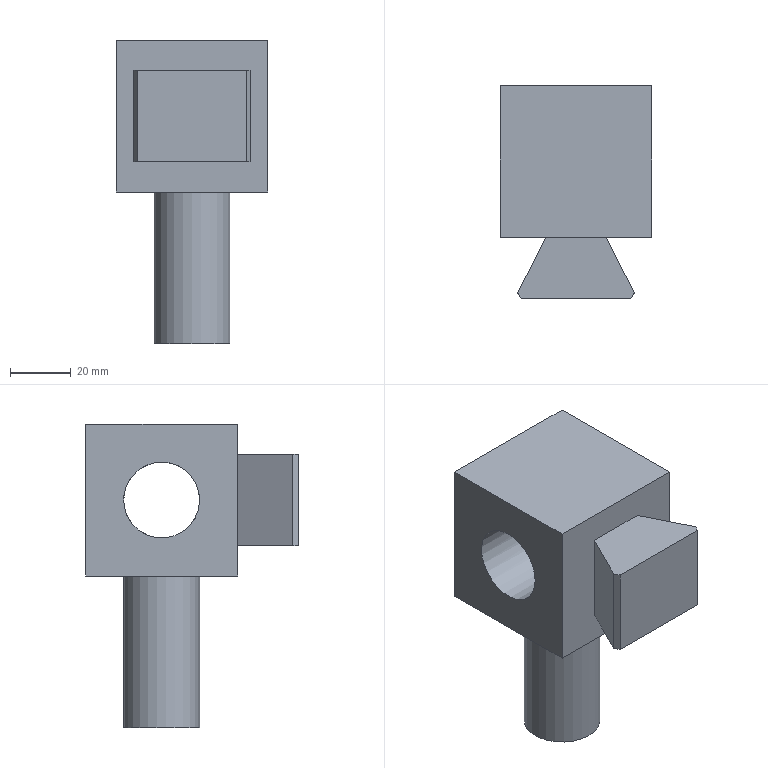Part | NX | features DATUM_CSYS 4, EXTRUDE 4, SKETCH 3, CHAMFER 1 | 1 solid | 16 faces | box 50 x 70 x 100 mm | volume 142893 mm3 | plane 14 | cylinder 2 | commonest cylinder face diameters 25 x2
STEP:
#1=CARTESIAN_POINT('',(-25.,0.,12.5));
#2=VERTEX_POINT('',#1);
#3=CARTESIAN_POINT('',(-25.,0.,0.));
#4=DIRECTION('',(-1.,0.,0.));
#5=DIRECTION('',(0.,0.,1.));
#6=AXIS2_PLACEMENT_3D('',#3,#4,#5);
#7=CIRCLE('',#6,12.5);
#8=EDGE_CURVE('',#2,#2,#7,.T.);
#9=ORIENTED_EDGE('',*,*,#8,.F.);
#10=EDGE_LOOP('',(#9));
#11=FACE_BOUND('',#10,.T.);
#12=CARTESIAN_POINT('',(-25.,25.,-25.));
#13=VERTEX_POINT('',#12);
#14=CARTESIAN_POINT('',(-25.,-25.,-25.));
#15=VERTEX_POINT('',#14);
#16=CARTESIAN_POINT('',(-25.,25.,-25.));
#17=DIRECTION('',(0.,-1.,0.));
#18=VECTOR('',#17,1000.);
#19=LINE('',#16,#18);
#20=EDGE_CURVE('',#13,#15,#19,.T.);
#21=ORIENTED_EDGE('',*,*,#20,.T.);
#22=CARTESIAN_POINT('',(-25.,-25.,25.));
#23=VERTEX_POINT('',#22);
#24=CARTESIAN_POINT('',(-25.,-25.,25.));
#25=DIRECTION('',(0.,0.,-1.));
#26=VECTOR('',#25,1000.);
#27=LINE('',#24,#26);
#28=EDGE_CURVE('',#23,#15,#27,.T.);
#29=ORIENTED_EDGE('',*,*,#28,.F.);
#30=CARTESIAN_POINT('',(-25.,25.,25.));
#31=VERTEX_POINT('',#30);
#32=CARTESIAN_POINT('',(-25.,25.,25.));
#33=DIRECTION('',(0.,-1.,0.));
#34=VECTOR('',#33,1000.);
#35=LINE('',#32,#34);
#36=EDGE_CURVE('',#31,#23,#35,.T.);
#37=ORIENTED_EDGE('',*,*,#36,.F.);
#38=CARTESIAN_POINT('',(-25.,25.,25.));
#39=DIRECTION('',(0.,0.,-1.));
#40=VECTOR('',#39,1000.);
#41=LINE('',#38,#40);
#42=EDGE_CURVE('',#31,#13,#41,.T.);
#43=ORIENTED_EDGE('',*,*,#42,.T.);
#44=EDGE_LOOP('',(#21,#29,#37,#43));
#45=FACE_BOUND('',#44,.T.);
#46=CARTESIAN_POINT('',(-25.,25.,25.));
#47=DIRECTION('',(1.,0.,0.));
#48=DIRECTION('',(0.,1.,0.));
#49=AXIS2_PLACEMENT_3D('',#46,#47,#48);
#50=PLANE('',#49);
#51=ADVANCED_FACE('',(#11,#45),#50,.F.);
#52=CARTESIAN_POINT('',(10.,-25.,15.));
#53=VERTEX_POINT('',#52);
#54=CARTESIAN_POINT('',(10.,-25.,-15.));
#55=VERTEX_POINT('',#54);
#56=CARTESIAN_POINT('',(10.,-25.,15.));
#57=DIRECTION('',(0.,0.,-1.));
#58=VECTOR('',#57,1000.);
#59=LINE('',#56,#58);
#60=EDGE_CURVE('',#53,#55,#59,.T.);
#61=ORIENTED_EDGE('',*,*,#60,.T.);
#62=CARTESIAN_POINT('',(-10.,-25.,-15.));
#63=VERTEX_POINT('',#62);
#64=CARTESIAN_POINT('',(10.,-25.,-15.));
#65=DIRECTION('',(-1.,0.,0.));
#66=VECTOR('',#65,1000.);
#67=LINE('',#64,#66);
#68=EDGE_CURVE('',#55,#63,#67,.T.);
#69=ORIENTED_EDGE('',*,*,#68,.T.);
#70=CARTESIAN_POINT('',(-10.,-25.,15.));
#71=VERTEX_POINT('',#70);
#72=CARTESIAN_POINT('',(-10.,-25.,15.));
#73=DIRECTION('',(0.,0.,-1.));
#74=VECTOR('',#73,1000.);
#75=LINE('',#72,#74);
#76=EDGE_CURVE('',#71,#63,#75,.T.);
#77=ORIENTED_EDGE('',*,*,#76,.F.);
#78=CARTESIAN_POINT('',(10.,-25.,15.));
#79=DIRECTION('',(-1.,0.,0.));
#80=VECTOR('',#79,1000.);
#81=LINE('',#78,#80);
#82=EDGE_CURVE('',#53,#71,#81,.T.);
#83=ORIENTED_EDGE('',*,*,#82,.F.);
#84=EDGE_LOOP('',(#61,#69,#77,#83));
#85=FACE_BOUND('',#84,.T.);
#86=CARTESIAN_POINT('',(25.,-25.,-25.));
#87=VERTEX_POINT('',#86);
#88=CARTESIAN_POINT('',(-25.,-25.,-25.));
#89=DIRECTION('',(1.,0.,0.));
#90=VECTOR('',#89,1000.);
#91=LINE('',#88,#90);
#92=EDGE_CURVE('',#15,#87,#91,.T.);
#93=ORIENTED_EDGE('',*,*,#92,.T.);
#94=CARTESIAN_POINT('',(25.,-25.,25.));
#95=VERTEX_POINT('',#94);
#96=CARTESIAN_POINT('',(25.,-25.,25.));
#97=DIRECTION('',(0.,0.,-1.));
#98=VECTOR('',#97,1000.);
#99=LINE('',#96,#98);
#100=EDGE_CURVE('',#95,#87,#99,.T.);
#101=ORIENTED_EDGE('',*,*,#100,.F.);
#102=CARTESIAN_POINT('',(-25.,-25.,25.));
#103=DIRECTION('',(1.,0.,0.));
#104=VECTOR('',#103,1000.);
#105=LINE('',#102,#104);
#106=EDGE_CURVE('',#23,#95,#105,.T.);
#107=ORIENTED_EDGE('',*,*,#106,.F.);
#108=ORIENTED_EDGE('',*,*,#28,.T.);
#109=EDGE_LOOP('',(#93,#101,#107,#108));
#110=FACE_BOUND('',#109,.T.);
#111=CARTESIAN_POINT('',(-25.,-25.,25.));
#112=DIRECTION('',(0.,1.,0.));
#113=DIRECTION('',(-1.,0.,0.));
#114=AXIS2_PLACEMENT_3D('',#111,#112,#113);
#115=PLANE('',#114);
#116=ADVANCED_FACE('',(#85,#110),#115,.F.);
#117=CARTESIAN_POINT('',(25.,-12.5,0.));
#118=VERTEX_POINT('',#117);
#119=CARTESIAN_POINT('',(25.,0.,0.));
#120=DIRECTION('',(-1.,0.,0.));
#121=DIRECTION('',(0.,-1.,0.));
#122=AXIS2_PLACEMENT_3D('',#119,#120,#121);
#123=CIRCLE('',#122,12.5);
#124=EDGE_CURVE('',#118,#118,#123,.T.);
#125=ORIENTED_EDGE('',*,*,#124,.T.);
#126=EDGE_LOOP('',(#125));
#127=FACE_BOUND('',#126,.T.);
#128=CARTESIAN_POINT('',(25.,25.,-25.));
#129=VERTEX_POINT('',#128);
#130=CARTESIAN_POINT('',(25.,-25.,-25.));
#131=DIRECTION('',(0.,1.,0.));
#132=VECTOR('',#131,1000.);
#133=LINE('',#130,#132);
#134=EDGE_CURVE('',#87,#129,#133,.T.);
#135=ORIENTED_EDGE('',*,*,#134,.T.);
#136=CARTESIAN_POINT('',(25.,25.,25.));
#137=VERTEX_POINT('',#136);
#138=CARTESIAN_POINT('',(25.,25.,25.));
#139=DIRECTION('',(0.,0.,-1.));
#140=VECTOR('',#139,1000.);
#141=LINE('',#138,#140);
#142=EDGE_CURVE('',#137,#129,#141,.T.);
#143=ORIENTED_EDGE('',*,*,#142,.F.);
#144=CARTESIAN_POINT('',(25.,-25.,25.));
#145=DIRECTION('',(0.,1.,0.));
#146=VECTOR('',#145,1000.);
#147=LINE('',#144,#146);
#148=EDGE_CURVE('',#95,#137,#147,.T.);
#149=ORIENTED_EDGE('',*,*,#148,.F.);
#150=ORIENTED_EDGE('',*,*,#100,.T.);
#151=EDGE_LOOP('',(#135,#143,#149,#150));
#152=FACE_BOUND('',#151,.T.);
#153=CARTESIAN_POINT('',(25.,-25.,25.));
#154=DIRECTION('',(-1.,0.,0.));
#155=DIRECTION('',(0.,-1.,0.));
#156=AXIS2_PLACEMENT_3D('',#153,#154,#155);
#157=PLANE('',#156);
#158=ADVANCED_FACE('',(#127,#152),#157,.F.);
#159=CARTESIAN_POINT('',(25.,25.,-25.));
#160=DIRECTION('',(-1.,0.,0.));
#161=VECTOR('',#160,1000.);
#162=LINE('',#159,#161);
#163=EDGE_CURVE('',#129,#13,#162,.T.);
#164=ORIENTED_EDGE('',*,*,#163,.T.);
#165=ORIENTED_EDGE('',*,*,#42,.F.);
#166=CARTESIAN_POINT('',(25.,25.,25.));
#167=DIRECTION('',(-1.,0.,0.));
#168=VECTOR('',#167,1000.);
#169=LINE('',#166,#168);
#170=EDGE_CURVE('',#137,#31,#169,.T.);
#171=ORIENTED_EDGE('',*,*,#170,.F.);
#172=ORIENTED_EDGE('',*,*,#142,.T.);
#173=EDGE_LOOP('',(#164,#165,#171,#172));
#174=FACE_BOUND('',#173,.T.);
#175=CARTESIAN_POINT('',(25.,25.,25.));
#176=DIRECTION('',(0.,-1.,0.));
#177=DIRECTION('',(0.,0.,-1.));
#178=AXIS2_PLACEMENT_3D('',#175,#176,#177);
#179=PLANE('',#178);
#180=ADVANCED_FACE('',(#174),#179,.F.);
#181=ORIENTED_EDGE('',*,*,#36,.T.);
#182=ORIENTED_EDGE('',*,*,#106,.T.);
#183=ORIENTED_EDGE('',*,*,#148,.T.);
#184=ORIENTED_EDGE('',*,*,#170,.T.);
#185=EDGE_LOOP('',(#181,#182,#183,#184));
#186=FACE_BOUND('',#185,.T.);
#187=CARTESIAN_POINT('',(0.,0.,25.));
#188=DIRECTION('',(0.,0.,1.));
#189=DIRECTION('',(1.,0.,0.));
#190=AXIS2_PLACEMENT_3D('',#187,#188,#189);
#191=PLANE('',#190);
#192=ADVANCED_FACE('',(#186),#191,.T.);
#193=CARTESIAN_POINT('',(0.,12.5,-25.));
#194=VERTEX_POINT('',#193);
#195=CARTESIAN_POINT('',(0.,0.,-25.));
#196=DIRECTION('',(0.,0.,-1.));
#197=DIRECTION('',(0.,1.,0.));
#198=AXIS2_PLACEMENT_3D('',#195,#196,#197);
#199=CIRCLE('',#198,12.5);
#200=EDGE_CURVE('',#194,#194,#199,.T.);
#201=ORIENTED_EDGE('',*,*,#200,.F.);
#202=EDGE_LOOP('',(#201));
#203=FACE_BOUND('',#202,.T.);
#204=ORIENTED_EDGE('',*,*,#20,.F.);
#205=ORIENTED_EDGE('',*,*,#163,.F.);
#206=ORIENTED_EDGE('',*,*,#134,.F.);
#207=ORIENTED_EDGE('',*,*,#92,.F.);
#208=EDGE_LOOP('',(#204,#205,#206,#207));
#209=FACE_BOUND('',#208,.T.);
#210=CARTESIAN_POINT('',(0.,0.,-25.));
#211=DIRECTION('',(0.,0.,1.));
#212=DIRECTION('',(1.,0.,0.));
#213=AXIS2_PLACEMENT_3D('',#210,#211,#212);
#214=PLANE('',#213);
#215=ADVANCED_FACE('',(#203,#209),#214,.F.);
#216=CARTESIAN_POINT('',(-19.106,-43.211,-15.));
#217=VERTEX_POINT('',#216);
#218=CARTESIAN_POINT('',(-10.,-25.,-15.));
#219=DIRECTION('',(-0.4472,-0.8944,0.));
#220=VECTOR('',#219,1000.);
#221=LINE('',#218,#220);
#222=EDGE_CURVE('',#63,#217,#221,.T.);
#223=ORIENTED_EDGE('',*,*,#222,.T.);
#224=CARTESIAN_POINT('',(-19.106,-43.211,15.));
#225=VERTEX_POINT('',#224);
#226=CARTESIAN_POINT('',(-19.106,-43.211,15.));
#227=DIRECTION('',(0.,0.,1.));
#228=VECTOR('',#227,1000.);
#229=LINE('',#226,#228);
#230=EDGE_CURVE('',#217,#225,#229,.T.);
#231=ORIENTED_EDGE('',*,*,#230,.T.);
#232=CARTESIAN_POINT('',(-10.,-25.,15.));
#233=DIRECTION('',(-0.4472,-0.8944,0.));
#234=VECTOR('',#233,1000.);
#235=LINE('',#232,#234);
#236=EDGE_CURVE('',#71,#225,#235,.T.);
#237=ORIENTED_EDGE('',*,*,#236,.F.);
#238=ORIENTED_EDGE('',*,*,#76,.T.);
#239=EDGE_LOOP('',(#223,#231,#237,#238));
#240=FACE_BOUND('',#239,.T.);
#241=CARTESIAN_POINT('',(-10.,-25.,15.));
#242=DIRECTION('',(0.8944,-0.4472,0.));
#243=DIRECTION('',(0.4472,0.8944,0.));
#244=AXIS2_PLACEMENT_3D('',#241,#242,#243);
#245=PLANE('',#244);
#246=ADVANCED_FACE('',(#240),#245,.F.);
#247=CARTESIAN_POINT('',(-18.,-45.,-15.));
#248=VERTEX_POINT('',#247);
#249=CARTESIAN_POINT('',(18.,-45.,-15.));
#250=VERTEX_POINT('',#249);
#251=CARTESIAN_POINT('',(0.,-45.,-15.));
#252=DIRECTION('',(1.,0.,0.));
#253=VECTOR('',#252,1000.);
#254=LINE('',#251,#253);
#255=EDGE_CURVE('',#248,#250,#254,.T.);
#256=ORIENTED_EDGE('',*,*,#255,.T.);
#257=CARTESIAN_POINT('',(18.,-45.,15.));
#258=VERTEX_POINT('',#257);
#259=CARTESIAN_POINT('',(18.,-45.,15.));
#260=DIRECTION('',(0.,0.,1.));
#261=VECTOR('',#260,1000.);
#262=LINE('',#259,#261);
#263=EDGE_CURVE('',#250,#258,#262,.T.);
#264=ORIENTED_EDGE('',*,*,#263,.T.);
#265=CARTESIAN_POINT('',(-18.,-45.,15.));
#266=VERTEX_POINT('',#265);
#267=CARTESIAN_POINT('',(-20.,-45.,15.));
#268=DIRECTION('',(1.,0.,0.));
#269=VECTOR('',#268,1000.);
#270=LINE('',#267,#269);
#271=EDGE_CURVE('',#266,#258,#270,.T.);
#272=ORIENTED_EDGE('',*,*,#271,.F.);
#273=CARTESIAN_POINT('',(-18.,-45.,15.));
#274=DIRECTION('',(0.,0.,-1.));
#275=VECTOR('',#274,1000.);
#276=LINE('',#273,#275);
#277=EDGE_CURVE('',#266,#248,#276,.T.);
#278=ORIENTED_EDGE('',*,*,#277,.T.);
#279=EDGE_LOOP('',(#256,#264,#272,#278));
#280=FACE_BOUND('',#279,.T.);
#281=CARTESIAN_POINT('',(0.,-45.,15.));
#282=DIRECTION('',(0.,1.,0.));
#283=DIRECTION('',(-1.,0.,0.));
#284=AXIS2_PLACEMENT_3D('',#281,#282,#283);
#285=PLANE('',#284);
#286=ADVANCED_FACE('',(#280),#285,.F.);
#287=CARTESIAN_POINT('',(19.106,-43.211,15.));
#288=VERTEX_POINT('',#287);
#289=CARTESIAN_POINT('',(20.,-45.,15.));
#290=DIRECTION('',(-0.4472,0.8944,0.));
#291=VECTOR('',#290,1000.);
#292=LINE('',#289,#291);
#293=EDGE_CURVE('',#288,#53,#292,.T.);
#294=ORIENTED_EDGE('',*,*,#293,.F.);
#295=CARTESIAN_POINT('',(19.106,-43.211,-15.));
#296=VERTEX_POINT('',#295);
#297=CARTESIAN_POINT('',(19.106,-43.211,15.));
#298=DIRECTION('',(0.,0.,-1.));
#299=VECTOR('',#298,1000.);
#300=LINE('',#297,#299);
#301=EDGE_CURVE('',#288,#296,#300,.T.);
#302=ORIENTED_EDGE('',*,*,#301,.T.);
#303=CARTESIAN_POINT('',(20.,-45.,-15.));
#304=DIRECTION('',(-0.4472,0.8944,0.));
#305=VECTOR('',#304,1000.);
#306=LINE('',#303,#305);
#307=EDGE_CURVE('',#296,#55,#306,.T.);
#308=ORIENTED_EDGE('',*,*,#307,.T.);
#309=ORIENTED_EDGE('',*,*,#60,.F.);
#310=EDGE_LOOP('',(#294,#302,#308,#309));
#311=FACE_BOUND('',#310,.T.);
#312=CARTESIAN_POINT('',(20.,-45.,15.));
#313=DIRECTION('',(-0.8944,-0.4472,0.));
#314=DIRECTION('',(0.4472,-0.8944,0.));
#315=AXIS2_PLACEMENT_3D('',#312,#313,#314);
#316=PLANE('',#315);
#317=ADVANCED_FACE('',(#311),#316,.F.);
#318=ORIENTED_EDGE('',*,*,#271,.T.);
#319=CARTESIAN_POINT('',(33.15,-20.488,15.));
#320=DIRECTION('',(-0.5257,-0.8507,0.));
#321=VECTOR('',#320,1000.);
#322=LINE('',#319,#321);
#323=EDGE_CURVE('',#258,#288,#322,.F.);
#324=ORIENTED_EDGE('',*,*,#323,.T.);
#325=ORIENTED_EDGE('',*,*,#293,.T.);
#326=ORIENTED_EDGE('',*,*,#82,.T.);
#327=ORIENTED_EDGE('',*,*,#236,.T.);
#328=CARTESIAN_POINT('',(-33.15,-20.488,15.));
#329=DIRECTION('',(-0.5257,0.8507,0.));
#330=VECTOR('',#329,1000.);
#331=LINE('',#328,#330);
#332=EDGE_CURVE('',#225,#266,#331,.F.);
#333=ORIENTED_EDGE('',*,*,#332,.T.);
#334=EDGE_LOOP('',(#318,#324,#325,#326,#327,#333));
#335=FACE_BOUND('',#334,.T.);
#336=CARTESIAN_POINT('',(0.,0.,15.));
#337=DIRECTION('',(0.,0.,1.));
#338=DIRECTION('',(1.,0.,0.));
#339=AXIS2_PLACEMENT_3D('',#336,#337,#338);
#340=PLANE('',#339);
#341=ADVANCED_FACE('',(#335),#340,.T.);
#342=ORIENTED_EDGE('',*,*,#307,.F.);
#343=CARTESIAN_POINT('',(19.106,-43.211,-15.));
#344=DIRECTION('',(0.5257,0.8507,0.));
#345=VECTOR('',#344,1000.);
#346=LINE('',#343,#345);
#347=EDGE_CURVE('',#296,#250,#346,.F.);
#348=ORIENTED_EDGE('',*,*,#347,.T.);
#349=ORIENTED_EDGE('',*,*,#255,.F.);
#350=CARTESIAN_POINT('',(-18.,-45.,-15.));
#351=DIRECTION('',(0.5257,-0.8507,0.));
#352=VECTOR('',#351,1000.);
#353=LINE('',#350,#352);
#354=EDGE_CURVE('',#248,#217,#353,.F.);
#355=ORIENTED_EDGE('',*,*,#354,.T.);
#356=ORIENTED_EDGE('',*,*,#222,.F.);
#357=ORIENTED_EDGE('',*,*,#68,.F.);
#358=EDGE_LOOP('',(#342,#348,#349,#355,#356,#357));
#359=FACE_BOUND('',#358,.T.);
#360=CARTESIAN_POINT('',(0.,0.,-15.));
#361=DIRECTION('',(0.,0.,1.));
#362=DIRECTION('',(1.,0.,0.));
#363=AXIS2_PLACEMENT_3D('',#360,#361,#362);
#364=PLANE('',#363);
#365=ADVANCED_FACE('',(#359),#364,.F.);
#366=ORIENTED_EDGE('',*,*,#323,.F.);
#367=ORIENTED_EDGE('',*,*,#263,.F.);
#368=ORIENTED_EDGE('',*,*,#347,.F.);
#369=ORIENTED_EDGE('',*,*,#301,.F.);
#370=EDGE_LOOP('',(#366,#367,#368,#369));
#371=FACE_BOUND('',#370,.T.);
#372=CARTESIAN_POINT('',(19.106,-43.211,15.));
#373=DIRECTION('',(-0.8507,0.5257,0.));
#374=DIRECTION('',(0.,0.,-1.));
#375=AXIS2_PLACEMENT_3D('',#372,#373,#374);
#376=PLANE('',#375);
#377=ADVANCED_FACE('',(#371),#376,.F.);
#378=ORIENTED_EDGE('',*,*,#332,.F.);
#379=ORIENTED_EDGE('',*,*,#230,.F.);
#380=ORIENTED_EDGE('',*,*,#354,.F.);
#381=ORIENTED_EDGE('',*,*,#277,.F.);
#382=EDGE_LOOP('',(#378,#379,#380,#381));
#383=FACE_BOUND('',#382,.T.);
#384=CARTESIAN_POINT('',(-18.,-45.,15.));
#385=DIRECTION('',(0.8507,0.5257,0.));
#386=DIRECTION('',(0.,0.,-1.));
#387=AXIS2_PLACEMENT_3D('',#384,#385,#386);
#388=PLANE('',#387);
#389=ADVANCED_FACE('',(#383),#388,.F.);
#390=ORIENTED_EDGE('',*,*,#8,.T.);
#391=EDGE_LOOP('',(#390));
#392=FACE_BOUND('',#391,.T.);
#393=ORIENTED_EDGE('',*,*,#124,.F.);
#394=EDGE_LOOP('',(#393));
#395=FACE_BOUND('',#394,.T.);
#396=CARTESIAN_POINT('',(75.,0.,0.));
#397=DIRECTION('',(-1.,0.,0.));
#398=DIRECTION('',(0.,-1.,0.));
#399=AXIS2_PLACEMENT_3D('',#396,#397,#398);
#400=CYLINDRICAL_SURFACE('',#399,12.5);
#401=ADVANCED_FACE('',(#392,#395),#400,.F.);
#402=CARTESIAN_POINT('',(0.,12.5,-75.));
#403=VERTEX_POINT('',#402);
#404=CARTESIAN_POINT('',(0.,0.,-75.));
#405=DIRECTION('',(0.,0.,-1.));
#406=DIRECTION('',(0.,1.,0.));
#407=AXIS2_PLACEMENT_3D('',#404,#405,#406);
#408=CIRCLE('',#407,12.5);
#409=EDGE_CURVE('',#403,#403,#408,.T.);
#410=ORIENTED_EDGE('',*,*,#409,.F.);
#411=EDGE_LOOP('',(#410));
#412=FACE_BOUND('',#411,.T.);
#413=ORIENTED_EDGE('',*,*,#200,.T.);
#414=EDGE_LOOP('',(#413));
#415=FACE_BOUND('',#414,.T.);
#416=CARTESIAN_POINT('',(0.,0.,-75.));
#417=DIRECTION('',(0.,0.,1.));
#418=DIRECTION('',(1.,0.,0.));
#419=AXIS2_PLACEMENT_3D('',#416,#417,#418);
#420=CYLINDRICAL_SURFACE('',#419,12.5);
#421=ADVANCED_FACE('',(#412,#415),#420,.T.);
#422=ORIENTED_EDGE('',*,*,#409,.T.);
#423=EDGE_LOOP('',(#422));
#424=FACE_BOUND('',#423,.T.);
#425=CARTESIAN_POINT('',(0.,0.,-75.));
#426=DIRECTION('',(0.,0.,-1.));
#427=DIRECTION('',(-1.,0.,0.));
#428=AXIS2_PLACEMENT_3D('',#425,#426,#427);
#429=PLANE('',#428);
#430=ADVANCED_FACE('',(#424),#429,.T.);
#431=CLOSED_SHELL('',(#51,#116,#158,#180,#192,#215,#246,#286,#317,#341,#365,#377,#389,#401,#421,#430));
#432=MANIFOLD_SOLID_BREP('',#431);
#433=(LENGTH_UNIT()NAMED_UNIT(*)SI_UNIT(.MILLI.,.METRE.));
#434=UNCERTAINTY_MEASURE_WITH_UNIT(LENGTH_MEASURE(0.00001),#433,'','');
#435=(NAMED_UNIT(*)PLANE_ANGLE_UNIT()SI_UNIT($,.RADIAN.));
#436=(NAMED_UNIT(*)SI_UNIT($,.STERADIAN.)SOLID_ANGLE_UNIT());
#437=(GEOMETRIC_REPRESENTATION_CONTEXT(3)GLOBAL_UNCERTAINTY_ASSIGNED_CONTEXT((#434))GLOBAL_UNIT_ASSIGNED_CONTEXT((#433,#435,#436))REPRESENTATION_CONTEXT('',''));
#438=ADVANCED_BREP_SHAPE_REPRESENTATION('',(#432),#437);